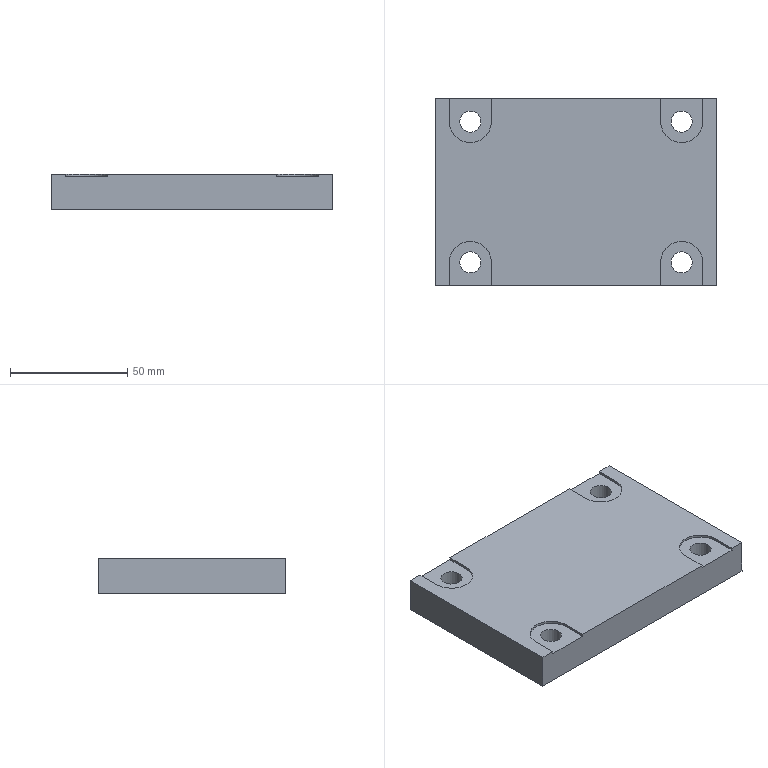Part | NX | 1 solid | 26 faces | box 120 x 80 x 15 mm | volume 139208 mm3 | plane 18 | cylinder 8 | commonest cylinder face diameters 9 x4 18 x4
STEP:
#1=CARTESIAN_POINT('',(-49.5,-30.,0.));
#2=VERTEX_POINT('',#1);
#3=CARTESIAN_POINT('',(-45.,-30.,0.));
#4=DIRECTION('',(0.,0.,1.));
#5=DIRECTION('',(-1.,0.,0.));
#6=AXIS2_PLACEMENT_3D('',#3,#4,#5);
#7=CIRCLE('',#6,4.5);
#8=EDGE_CURVE('',#2,#2,#7,.T.);
#9=ORIENTED_EDGE('',*,*,#8,.F.);
#10=EDGE_LOOP('',(#9));
#11=FACE_BOUND('',#10,.T.);
#12=CARTESIAN_POINT('',(-40.5,-30.,14.));
#13=VERTEX_POINT('',#12);
#14=CARTESIAN_POINT('',(-45.,-30.,14.));
#15=DIRECTION('',(0.,0.,1.));
#16=DIRECTION('',(1.,0.,0.));
#17=AXIS2_PLACEMENT_3D('',#14,#15,#16);
#18=CIRCLE('',#17,4.5);
#19=EDGE_CURVE('',#13,#13,#18,.F.);
#20=ORIENTED_EDGE('',*,*,#19,.F.);
#21=EDGE_LOOP('',(#20));
#22=FACE_BOUND('',#21,.T.);
#23=CARTESIAN_POINT('',(-45.,-30.,0.));
#24=DIRECTION('',(0.,0.,1.));
#25=DIRECTION('',(1.,0.,0.));
#26=AXIS2_PLACEMENT_3D('',#23,#24,#25);
#27=CYLINDRICAL_SURFACE('',#26,4.5);
#28=ADVANCED_FACE('',(#11,#22),#27,.F.);
#29=CARTESIAN_POINT('',(49.5,-30.,0.));
#30=VERTEX_POINT('',#29);
#31=CARTESIAN_POINT('',(45.,-30.,0.));
#32=DIRECTION('',(0.,0.,1.));
#33=DIRECTION('',(1.,0.,0.));
#34=AXIS2_PLACEMENT_3D('',#31,#32,#33);
#35=CIRCLE('',#34,4.5);
#36=EDGE_CURVE('',#30,#30,#35,.T.);
#37=ORIENTED_EDGE('',*,*,#36,.F.);
#38=EDGE_LOOP('',(#37));
#39=FACE_BOUND('',#38,.T.);
#40=CARTESIAN_POINT('',(49.5,-30.,14.));
#41=VERTEX_POINT('',#40);
#42=CARTESIAN_POINT('',(45.,-30.,14.));
#43=DIRECTION('',(0.,0.,1.));
#44=DIRECTION('',(1.,0.,0.));
#45=AXIS2_PLACEMENT_3D('',#42,#43,#44);
#46=CIRCLE('',#45,4.5);
#47=EDGE_CURVE('',#41,#41,#46,.F.);
#48=ORIENTED_EDGE('',*,*,#47,.F.);
#49=EDGE_LOOP('',(#48));
#50=FACE_BOUND('',#49,.T.);
#51=CARTESIAN_POINT('',(45.,-30.,0.));
#52=DIRECTION('',(0.,0.,1.));
#53=DIRECTION('',(1.,0.,0.));
#54=AXIS2_PLACEMENT_3D('',#51,#52,#53);
#55=CYLINDRICAL_SURFACE('',#54,4.5);
#56=ADVANCED_FACE('',(#39,#50),#55,.F.);
#57=CARTESIAN_POINT('',(40.5,30.,0.));
#58=VERTEX_POINT('',#57);
#59=CARTESIAN_POINT('',(45.,30.,0.));
#60=DIRECTION('',(0.,0.,1.));
#61=DIRECTION('',(-1.,0.,0.));
#62=AXIS2_PLACEMENT_3D('',#59,#60,#61);
#63=CIRCLE('',#62,4.5);
#64=EDGE_CURVE('',#58,#58,#63,.T.);
#65=ORIENTED_EDGE('',*,*,#64,.F.);
#66=EDGE_LOOP('',(#65));
#67=FACE_BOUND('',#66,.T.);
#68=CARTESIAN_POINT('',(49.5,30.,14.));
#69=VERTEX_POINT('',#68);
#70=CARTESIAN_POINT('',(45.,30.,14.));
#71=DIRECTION('',(0.,0.,1.));
#72=DIRECTION('',(1.,0.,0.));
#73=AXIS2_PLACEMENT_3D('',#70,#71,#72);
#74=CIRCLE('',#73,4.5);
#75=EDGE_CURVE('',#69,#69,#74,.F.);
#76=ORIENTED_EDGE('',*,*,#75,.F.);
#77=EDGE_LOOP('',(#76));
#78=FACE_BOUND('',#77,.T.);
#79=CARTESIAN_POINT('',(45.,30.,0.));
#80=DIRECTION('',(0.,0.,1.));
#81=DIRECTION('',(1.,0.,0.));
#82=AXIS2_PLACEMENT_3D('',#79,#80,#81);
#83=CYLINDRICAL_SURFACE('',#82,4.5);
#84=ADVANCED_FACE('',(#67,#78),#83,.F.);
#85=CARTESIAN_POINT('',(-40.5,30.,0.));
#86=VERTEX_POINT('',#85);
#87=CARTESIAN_POINT('',(-45.,30.,0.));
#88=DIRECTION('',(0.,0.,1.));
#89=DIRECTION('',(1.,0.,0.));
#90=AXIS2_PLACEMENT_3D('',#87,#88,#89);
#91=CIRCLE('',#90,4.5);
#92=EDGE_CURVE('',#86,#86,#91,.T.);
#93=ORIENTED_EDGE('',*,*,#92,.F.);
#94=EDGE_LOOP('',(#93));
#95=FACE_BOUND('',#94,.T.);
#96=CARTESIAN_POINT('',(-40.5,30.,14.));
#97=VERTEX_POINT('',#96);
#98=CARTESIAN_POINT('',(-45.,30.,14.));
#99=DIRECTION('',(0.,0.,1.));
#100=DIRECTION('',(1.,0.,0.));
#101=AXIS2_PLACEMENT_3D('',#98,#99,#100);
#102=CIRCLE('',#101,4.5);
#103=EDGE_CURVE('',#97,#97,#102,.F.);
#104=ORIENTED_EDGE('',*,*,#103,.F.);
#105=EDGE_LOOP('',(#104));
#106=FACE_BOUND('',#105,.T.);
#107=CARTESIAN_POINT('',(-45.,30.,0.));
#108=DIRECTION('',(0.,0.,1.));
#109=DIRECTION('',(1.,0.,0.));
#110=AXIS2_PLACEMENT_3D('',#107,#108,#109);
#111=CYLINDRICAL_SURFACE('',#110,4.5);
#112=ADVANCED_FACE('',(#95,#106),#111,.F.);
#113=CARTESIAN_POINT('',(60.,-40.,0.));
#114=VERTEX_POINT('',#113);
#115=CARTESIAN_POINT('',(60.,40.,0.));
#116=VERTEX_POINT('',#115);
#117=CARTESIAN_POINT('',(60.,-40.,0.));
#118=DIRECTION('',(0.,1.,0.));
#119=VECTOR('',#118,1000.);
#120=LINE('',#117,#119);
#121=EDGE_CURVE('',#114,#116,#120,.T.);
#122=ORIENTED_EDGE('',*,*,#121,.T.);
#123=CARTESIAN_POINT('',(60.,40.,15.));
#124=VERTEX_POINT('',#123);
#125=CARTESIAN_POINT('',(60.,40.,15.));
#126=DIRECTION('',(0.,0.,-1.));
#127=VECTOR('',#126,1000.);
#128=LINE('',#125,#127);
#129=EDGE_CURVE('',#124,#116,#128,.T.);
#130=ORIENTED_EDGE('',*,*,#129,.F.);
#131=CARTESIAN_POINT('',(60.,-40.,15.));
#132=VERTEX_POINT('',#131);
#133=CARTESIAN_POINT('',(60.,-40.,15.));
#134=DIRECTION('',(0.,1.,0.));
#135=VECTOR('',#134,1000.);
#136=LINE('',#133,#135);
#137=EDGE_CURVE('',#132,#124,#136,.T.);
#138=ORIENTED_EDGE('',*,*,#137,.F.);
#139=CARTESIAN_POINT('',(60.,-40.,15.));
#140=DIRECTION('',(0.,0.,-1.));
#141=VECTOR('',#140,1000.);
#142=LINE('',#139,#141);
#143=EDGE_CURVE('',#132,#114,#142,.T.);
#144=ORIENTED_EDGE('',*,*,#143,.T.);
#145=EDGE_LOOP('',(#122,#130,#138,#144));
#146=FACE_BOUND('',#145,.T.);
#147=CARTESIAN_POINT('',(60.,-40.,15.));
#148=DIRECTION('',(-1.,0.,0.));
#149=DIRECTION('',(0.,0.,1.));
#150=AXIS2_PLACEMENT_3D('',#147,#148,#149);
#151=PLANE('',#150);
#152=ADVANCED_FACE('',(#146),#151,.F.);
#153=CARTESIAN_POINT('',(36.,40.,15.));
#154=VERTEX_POINT('',#153);
#155=CARTESIAN_POINT('',(-36.,40.,15.));
#156=VERTEX_POINT('',#155);
#157=CARTESIAN_POINT('',(-60.,40.,15.));
#158=DIRECTION('',(-1.,0.,0.));
#159=VECTOR('',#158,1000.);
#160=LINE('',#157,#159);
#161=EDGE_CURVE('',#154,#156,#160,.T.);
#162=ORIENTED_EDGE('',*,*,#161,.F.);
#163=CARTESIAN_POINT('',(36.,40.,14.));
#164=VERTEX_POINT('',#163);
#165=CARTESIAN_POINT('',(36.,40.,14.));
#166=DIRECTION('',(0.,0.,1.));
#167=VECTOR('',#166,1000.);
#168=LINE('',#165,#167);
#169=EDGE_CURVE('',#164,#154,#168,.T.);
#170=ORIENTED_EDGE('',*,*,#169,.F.);
#171=CARTESIAN_POINT('',(54.,40.,14.));
#172=VERTEX_POINT('',#171);
#173=CARTESIAN_POINT('',(-60.,40.,14.));
#174=DIRECTION('',(-1.,0.,0.));
#175=VECTOR('',#174,1000.);
#176=LINE('',#173,#175);
#177=EDGE_CURVE('',#172,#164,#176,.T.);
#178=ORIENTED_EDGE('',*,*,#177,.F.);
#179=CARTESIAN_POINT('',(54.,40.,15.));
#180=VERTEX_POINT('',#179);
#181=CARTESIAN_POINT('',(54.,40.,14.));
#182=DIRECTION('',(0.,0.,1.));
#183=VECTOR('',#182,1000.);
#184=LINE('',#181,#183);
#185=EDGE_CURVE('',#172,#180,#184,.T.);
#186=ORIENTED_EDGE('',*,*,#185,.T.);
#187=CARTESIAN_POINT('',(-60.,40.,15.));
#188=DIRECTION('',(-1.,0.,0.));
#189=VECTOR('',#188,1000.);
#190=LINE('',#187,#189);
#191=EDGE_CURVE('',#124,#180,#190,.T.);
#192=ORIENTED_EDGE('',*,*,#191,.F.);
#193=ORIENTED_EDGE('',*,*,#129,.T.);
#194=CARTESIAN_POINT('',(-60.,40.,0.));
#195=VERTEX_POINT('',#194);
#196=CARTESIAN_POINT('',(-60.,40.,0.));
#197=DIRECTION('',(-1.,0.,0.));
#198=VECTOR('',#197,1000.);
#199=LINE('',#196,#198);
#200=EDGE_CURVE('',#116,#195,#199,.T.);
#201=ORIENTED_EDGE('',*,*,#200,.T.);
#202=CARTESIAN_POINT('',(-60.,40.,15.));
#203=VERTEX_POINT('',#202);
#204=CARTESIAN_POINT('',(-60.,40.,15.));
#205=DIRECTION('',(0.,0.,-1.));
#206=VECTOR('',#205,1000.);
#207=LINE('',#204,#206);
#208=EDGE_CURVE('',#203,#195,#207,.T.);
#209=ORIENTED_EDGE('',*,*,#208,.F.);
#210=CARTESIAN_POINT('',(-54.,40.,15.));
#211=VERTEX_POINT('',#210);
#212=CARTESIAN_POINT('',(-60.,40.,15.));
#213=DIRECTION('',(-1.,0.,0.));
#214=VECTOR('',#213,1000.);
#215=LINE('',#212,#214);
#216=EDGE_CURVE('',#211,#203,#215,.T.);
#217=ORIENTED_EDGE('',*,*,#216,.F.);
#218=CARTESIAN_POINT('',(-54.,40.,14.));
#219=VERTEX_POINT('',#218);
#220=CARTESIAN_POINT('',(-54.,40.,14.));
#221=DIRECTION('',(0.,0.,1.));
#222=VECTOR('',#221,1000.);
#223=LINE('',#220,#222);
#224=EDGE_CURVE('',#219,#211,#223,.T.);
#225=ORIENTED_EDGE('',*,*,#224,.F.);
#226=CARTESIAN_POINT('',(-36.,40.,14.));
#227=VERTEX_POINT('',#226);
#228=CARTESIAN_POINT('',(-60.,40.,14.));
#229=DIRECTION('',(-1.,0.,0.));
#230=VECTOR('',#229,1000.);
#231=LINE('',#228,#230);
#232=EDGE_CURVE('',#227,#219,#231,.T.);
#233=ORIENTED_EDGE('',*,*,#232,.F.);
#234=CARTESIAN_POINT('',(-36.,40.,14.));
#235=DIRECTION('',(0.,0.,1.));
#236=VECTOR('',#235,1000.);
#237=LINE('',#234,#236);
#238=EDGE_CURVE('',#227,#156,#237,.T.);
#239=ORIENTED_EDGE('',*,*,#238,.T.);
#240=EDGE_LOOP('',(#162,#170,#178,#186,#192,#193,#201,#209,#217,#225,#233,#239));
#241=FACE_BOUND('',#240,.T.);
#242=CARTESIAN_POINT('',(-60.,40.,15.));
#243=DIRECTION('',(0.,-1.,0.));
#244=DIRECTION('',(0.,0.,-1.));
#245=AXIS2_PLACEMENT_3D('',#242,#243,#244);
#246=PLANE('',#245);
#247=ADVANCED_FACE('',(#241),#246,.F.);
#248=CARTESIAN_POINT('',(-60.,-40.,0.));
#249=VERTEX_POINT('',#248);
#250=CARTESIAN_POINT('',(-60.,-40.,0.));
#251=DIRECTION('',(0.,-1.,0.));
#252=VECTOR('',#251,1000.);
#253=LINE('',#250,#252);
#254=EDGE_CURVE('',#195,#249,#253,.T.);
#255=ORIENTED_EDGE('',*,*,#254,.T.);
#256=CARTESIAN_POINT('',(-60.,-40.,15.));
#257=VERTEX_POINT('',#256);
#258=CARTESIAN_POINT('',(-60.,-40.,15.));
#259=DIRECTION('',(0.,0.,-1.));
#260=VECTOR('',#259,1000.);
#261=LINE('',#258,#260);
#262=EDGE_CURVE('',#257,#249,#261,.T.);
#263=ORIENTED_EDGE('',*,*,#262,.F.);
#264=CARTESIAN_POINT('',(-60.,-40.,15.));
#265=DIRECTION('',(0.,-1.,0.));
#266=VECTOR('',#265,1000.);
#267=LINE('',#264,#266);
#268=EDGE_CURVE('',#203,#257,#267,.T.);
#269=ORIENTED_EDGE('',*,*,#268,.F.);
#270=ORIENTED_EDGE('',*,*,#208,.T.);
#271=EDGE_LOOP('',(#255,#263,#269,#270));
#272=FACE_BOUND('',#271,.T.);
#273=CARTESIAN_POINT('',(-60.,-40.,15.));
#274=DIRECTION('',(1.,0.,0.));
#275=DIRECTION('',(0.,0.,-1.));
#276=AXIS2_PLACEMENT_3D('',#273,#274,#275);
#277=PLANE('',#276);
#278=ADVANCED_FACE('',(#272),#277,.F.);
#279=CARTESIAN_POINT('',(-36.,-40.,15.));
#280=VERTEX_POINT('',#279);
#281=CARTESIAN_POINT('',(36.,-40.,15.));
#282=VERTEX_POINT('',#281);
#283=CARTESIAN_POINT('',(-60.,-40.,15.));
#284=DIRECTION('',(1.,0.,0.));
#285=VECTOR('',#284,1000.);
#286=LINE('',#283,#285);
#287=EDGE_CURVE('',#280,#282,#286,.T.);
#288=ORIENTED_EDGE('',*,*,#287,.F.);
#289=CARTESIAN_POINT('',(-36.,-40.,14.));
#290=VERTEX_POINT('',#289);
#291=CARTESIAN_POINT('',(-36.,-40.,14.));
#292=DIRECTION('',(0.,0.,1.));
#293=VECTOR('',#292,1000.);
#294=LINE('',#291,#293);
#295=EDGE_CURVE('',#290,#280,#294,.T.);
#296=ORIENTED_EDGE('',*,*,#295,.F.);
#297=CARTESIAN_POINT('',(-54.,-40.,14.));
#298=VERTEX_POINT('',#297);
#299=CARTESIAN_POINT('',(-60.,-40.,14.));
#300=DIRECTION('',(1.,0.,0.));
#301=VECTOR('',#300,1000.);
#302=LINE('',#299,#301);
#303=EDGE_CURVE('',#298,#290,#302,.T.);
#304=ORIENTED_EDGE('',*,*,#303,.F.);
#305=CARTESIAN_POINT('',(-54.,-40.,15.));
#306=VERTEX_POINT('',#305);
#307=CARTESIAN_POINT('',(-54.,-40.,14.));
#308=DIRECTION('',(0.,0.,1.));
#309=VECTOR('',#308,1000.);
#310=LINE('',#307,#309);
#311=EDGE_CURVE('',#298,#306,#310,.T.);
#312=ORIENTED_EDGE('',*,*,#311,.T.);
#313=CARTESIAN_POINT('',(-60.,-40.,15.));
#314=DIRECTION('',(1.,0.,0.));
#315=VECTOR('',#314,1000.);
#316=LINE('',#313,#315);
#317=EDGE_CURVE('',#257,#306,#316,.T.);
#318=ORIENTED_EDGE('',*,*,#317,.F.);
#319=ORIENTED_EDGE('',*,*,#262,.T.);
#320=CARTESIAN_POINT('',(-60.,-40.,0.));
#321=DIRECTION('',(1.,0.,0.));
#322=VECTOR('',#321,1000.);
#323=LINE('',#320,#322);
#324=EDGE_CURVE('',#249,#114,#323,.T.);
#325=ORIENTED_EDGE('',*,*,#324,.T.);
#326=ORIENTED_EDGE('',*,*,#143,.F.);
#327=CARTESIAN_POINT('',(54.,-40.,15.));
#328=VERTEX_POINT('',#327);
#329=CARTESIAN_POINT('',(-60.,-40.,15.));
#330=DIRECTION('',(1.,0.,0.));
#331=VECTOR('',#330,1000.);
#332=LINE('',#329,#331);
#333=EDGE_CURVE('',#328,#132,#332,.T.);
#334=ORIENTED_EDGE('',*,*,#333,.F.);
#335=CARTESIAN_POINT('',(54.,-40.,14.));
#336=VERTEX_POINT('',#335);
#337=CARTESIAN_POINT('',(54.,-40.,14.));
#338=DIRECTION('',(0.,0.,1.));
#339=VECTOR('',#338,1000.);
#340=LINE('',#337,#339);
#341=EDGE_CURVE('',#336,#328,#340,.T.);
#342=ORIENTED_EDGE('',*,*,#341,.F.);
#343=CARTESIAN_POINT('',(36.,-40.,14.));
#344=VERTEX_POINT('',#343);
#345=CARTESIAN_POINT('',(-60.,-40.,14.));
#346=DIRECTION('',(1.,0.,0.));
#347=VECTOR('',#346,1000.);
#348=LINE('',#345,#347);
#349=EDGE_CURVE('',#344,#336,#348,.T.);
#350=ORIENTED_EDGE('',*,*,#349,.F.);
#351=CARTESIAN_POINT('',(36.,-40.,14.));
#352=DIRECTION('',(0.,0.,1.));
#353=VECTOR('',#352,1000.);
#354=LINE('',#351,#353);
#355=EDGE_CURVE('',#344,#282,#354,.T.);
#356=ORIENTED_EDGE('',*,*,#355,.T.);
#357=EDGE_LOOP('',(#288,#296,#304,#312,#318,#319,#325,#326,#334,#342,#350,#356));
#358=FACE_BOUND('',#357,.T.);
#359=CARTESIAN_POINT('',(-60.,-40.,15.));
#360=DIRECTION('',(0.,1.,0.));
#361=DIRECTION('',(0.,0.,1.));
#362=AXIS2_PLACEMENT_3D('',#359,#360,#361);
#363=PLANE('',#362);
#364=ADVANCED_FACE('',(#358),#363,.F.);
#365=CARTESIAN_POINT('',(-36.,-30.,15.));
#366=VERTEX_POINT('',#365);
#367=CARTESIAN_POINT('',(-54.,-30.,15.));
#368=VERTEX_POINT('',#367);
#369=CARTESIAN_POINT('',(-45.,-30.,15.));
#370=DIRECTION('',(0.,0.,1.));
#371=DIRECTION('',(1.,0.,0.));
#372=AXIS2_PLACEMENT_3D('',#369,#370,#371);
#373=CIRCLE('',#372,9.);
#374=EDGE_CURVE('',#366,#368,#373,.T.);
#375=ORIENTED_EDGE('',*,*,#374,.F.);
#376=CARTESIAN_POINT('',(-36.,-30.,15.));
#377=DIRECTION('',(0.,1.,0.));
#378=VECTOR('',#377,1000.);
#379=LINE('',#376,#378);
#380=EDGE_CURVE('',#280,#366,#379,.T.);
#381=ORIENTED_EDGE('',*,*,#380,.F.);
#382=ORIENTED_EDGE('',*,*,#287,.T.);
#383=CARTESIAN_POINT('',(36.,-30.,15.));
#384=VERTEX_POINT('',#383);
#385=CARTESIAN_POINT('',(36.,-30.,15.));
#386=DIRECTION('',(0.,-1.,0.));
#387=VECTOR('',#386,1000.);
#388=LINE('',#385,#387);
#389=EDGE_CURVE('',#384,#282,#388,.T.);
#390=ORIENTED_EDGE('',*,*,#389,.F.);
#391=CARTESIAN_POINT('',(54.,-30.,15.));
#392=VERTEX_POINT('',#391);
#393=CARTESIAN_POINT('',(45.,-30.,15.));
#394=DIRECTION('',(0.,0.,1.));
#395=DIRECTION('',(1.,0.,0.));
#396=AXIS2_PLACEMENT_3D('',#393,#394,#395);
#397=CIRCLE('',#396,9.);
#398=EDGE_CURVE('',#392,#384,#397,.T.);
#399=ORIENTED_EDGE('',*,*,#398,.F.);
#400=CARTESIAN_POINT('',(54.,-30.,15.));
#401=DIRECTION('',(0.,1.,0.));
#402=VECTOR('',#401,1000.);
#403=LINE('',#400,#402);
#404=EDGE_CURVE('',#328,#392,#403,.T.);
#405=ORIENTED_EDGE('',*,*,#404,.F.);
#406=ORIENTED_EDGE('',*,*,#333,.T.);
#407=ORIENTED_EDGE('',*,*,#137,.T.);
#408=ORIENTED_EDGE('',*,*,#191,.T.);
#409=CARTESIAN_POINT('',(54.,30.,15.));
#410=VERTEX_POINT('',#409);
#411=CARTESIAN_POINT('',(54.,30.,15.));
#412=DIRECTION('',(0.,1.,0.));
#413=VECTOR('',#412,1000.);
#414=LINE('',#411,#413);
#415=EDGE_CURVE('',#410,#180,#414,.T.);
#416=ORIENTED_EDGE('',*,*,#415,.F.);
#417=CARTESIAN_POINT('',(36.,30.,15.));
#418=VERTEX_POINT('',#417);
#419=CARTESIAN_POINT('',(45.,30.,15.));
#420=DIRECTION('',(0.,0.,1.));
#421=DIRECTION('',(1.,0.,0.));
#422=AXIS2_PLACEMENT_3D('',#419,#420,#421);
#423=CIRCLE('',#422,9.);
#424=EDGE_CURVE('',#418,#410,#423,.T.);
#425=ORIENTED_EDGE('',*,*,#424,.F.);
#426=CARTESIAN_POINT('',(36.,30.,15.));
#427=DIRECTION('',(0.,-1.,0.));
#428=VECTOR('',#427,1000.);
#429=LINE('',#426,#428);
#430=EDGE_CURVE('',#154,#418,#429,.T.);
#431=ORIENTED_EDGE('',*,*,#430,.F.);
#432=ORIENTED_EDGE('',*,*,#161,.T.);
#433=CARTESIAN_POINT('',(-36.,30.,15.));
#434=VERTEX_POINT('',#433);
#435=CARTESIAN_POINT('',(-36.,30.,15.));
#436=DIRECTION('',(0.,1.,0.));
#437=VECTOR('',#436,1000.);
#438=LINE('',#435,#437);
#439=EDGE_CURVE('',#434,#156,#438,.T.);
#440=ORIENTED_EDGE('',*,*,#439,.F.);
#441=CARTESIAN_POINT('',(-54.,30.,15.));
#442=VERTEX_POINT('',#441);
#443=CARTESIAN_POINT('',(-45.,30.,15.));
#444=DIRECTION('',(0.,0.,1.));
#445=DIRECTION('',(1.,0.,0.));
#446=AXIS2_PLACEMENT_3D('',#443,#444,#445);
#447=CIRCLE('',#446,9.);
#448=EDGE_CURVE('',#442,#434,#447,.T.);
#449=ORIENTED_EDGE('',*,*,#448,.F.);
#450=CARTESIAN_POINT('',(-54.,30.,15.));
#451=DIRECTION('',(0.,-1.,0.));
#452=VECTOR('',#451,1000.);
#453=LINE('',#450,#452);
#454=EDGE_CURVE('',#211,#442,#453,.T.);
#455=ORIENTED_EDGE('',*,*,#454,.F.);
#456=ORIENTED_EDGE('',*,*,#216,.T.);
#457=ORIENTED_EDGE('',*,*,#268,.T.);
#458=ORIENTED_EDGE('',*,*,#317,.T.);
#459=CARTESIAN_POINT('',(-54.,-30.,15.));
#460=DIRECTION('',(0.,-1.,0.));
#461=VECTOR('',#460,1000.);
#462=LINE('',#459,#461);
#463=EDGE_CURVE('',#368,#306,#462,.T.);
#464=ORIENTED_EDGE('',*,*,#463,.F.);
#465=EDGE_LOOP('',(#375,#381,#382,#390,#399,#405,#406,#407,#408,#416,#425,#431,#432,#440,#449,#455,#456,#457,#458,#464));
#466=FACE_BOUND('',#465,.T.);
#467=CARTESIAN_POINT('',(0.,0.,15.));
#468=DIRECTION('',(0.,0.,-1.));
#469=DIRECTION('',(-1.,0.,0.));
#470=AXIS2_PLACEMENT_3D('',#467,#468,#469);
#471=PLANE('',#470);
#472=ADVANCED_FACE('',(#466),#471,.F.);
#473=ORIENTED_EDGE('',*,*,#8,.T.);
#474=EDGE_LOOP('',(#473));
#475=FACE_BOUND('',#474,.T.);
#476=ORIENTED_EDGE('',*,*,#36,.T.);
#477=EDGE_LOOP('',(#476));
#478=FACE_BOUND('',#477,.T.);
#479=ORIENTED_EDGE('',*,*,#64,.T.);
#480=EDGE_LOOP('',(#479));
#481=FACE_BOUND('',#480,.T.);
#482=ORIENTED_EDGE('',*,*,#92,.T.);
#483=EDGE_LOOP('',(#482));
#484=FACE_BOUND('',#483,.T.);
#485=ORIENTED_EDGE('',*,*,#121,.F.);
#486=ORIENTED_EDGE('',*,*,#324,.F.);
#487=ORIENTED_EDGE('',*,*,#254,.F.);
#488=ORIENTED_EDGE('',*,*,#200,.F.);
#489=EDGE_LOOP('',(#485,#486,#487,#488));
#490=FACE_BOUND('',#489,.T.);
#491=CARTESIAN_POINT('',(0.,0.,0.));
#492=DIRECTION('',(0.,0.,-1.));
#493=DIRECTION('',(-1.,0.,0.));
#494=AXIS2_PLACEMENT_3D('',#491,#492,#493);
#495=PLANE('',#494);
#496=ADVANCED_FACE('',(#475,#478,#481,#484,#490),#495,.T.);
#497=ORIENTED_EDGE('',*,*,#103,.T.);
#498=EDGE_LOOP('',(#497));
#499=FACE_BOUND('',#498,.T.);
#500=ORIENTED_EDGE('',*,*,#232,.T.);
#501=CARTESIAN_POINT('',(-54.,30.,14.));
#502=VERTEX_POINT('',#501);
#503=CARTESIAN_POINT('',(-54.,30.,14.));
#504=DIRECTION('',(0.,-1.,0.));
#505=VECTOR('',#504,1000.);
#506=LINE('',#503,#505);
#507=EDGE_CURVE('',#219,#502,#506,.T.);
#508=ORIENTED_EDGE('',*,*,#507,.T.);
#509=CARTESIAN_POINT('',(-36.,30.,14.));
#510=VERTEX_POINT('',#509);
#511=CARTESIAN_POINT('',(-45.,30.,14.));
#512=DIRECTION('',(0.,0.,1.));
#513=DIRECTION('',(1.,0.,0.));
#514=AXIS2_PLACEMENT_3D('',#511,#512,#513);
#515=CIRCLE('',#514,9.);
#516=EDGE_CURVE('',#502,#510,#515,.T.);
#517=ORIENTED_EDGE('',*,*,#516,.T.);
#518=CARTESIAN_POINT('',(-36.,30.,14.));
#519=DIRECTION('',(0.,1.,0.));
#520=VECTOR('',#519,1000.);
#521=LINE('',#518,#520);
#522=EDGE_CURVE('',#510,#227,#521,.T.);
#523=ORIENTED_EDGE('',*,*,#522,.T.);
#524=EDGE_LOOP('',(#500,#508,#517,#523));
#525=FACE_BOUND('',#524,.T.);
#526=CARTESIAN_POINT('',(-45.,30.,14.));
#527=DIRECTION('',(0.,0.,1.));
#528=DIRECTION('',(1.,0.,0.));
#529=AXIS2_PLACEMENT_3D('',#526,#527,#528);
#530=PLANE('',#529);
#531=ADVANCED_FACE('',(#499,#525),#530,.T.);
#532=ORIENTED_EDGE('',*,*,#448,.T.);
#533=CARTESIAN_POINT('',(-36.,30.,14.));
#534=DIRECTION('',(0.,0.,1.));
#535=VECTOR('',#534,1000.);
#536=LINE('',#533,#535);
#537=EDGE_CURVE('',#510,#434,#536,.T.);
#538=ORIENTED_EDGE('',*,*,#537,.F.);
#539=ORIENTED_EDGE('',*,*,#516,.F.);
#540=CARTESIAN_POINT('',(-54.,30.,14.));
#541=DIRECTION('',(0.,0.,1.));
#542=VECTOR('',#541,1000.);
#543=LINE('',#540,#542);
#544=EDGE_CURVE('',#502,#442,#543,.T.);
#545=ORIENTED_EDGE('',*,*,#544,.T.);
#546=EDGE_LOOP('',(#532,#538,#539,#545));
#547=FACE_BOUND('',#546,.T.);
#548=CARTESIAN_POINT('',(-45.,30.,14.));
#549=DIRECTION('',(0.,0.,1.));
#550=DIRECTION('',(1.,0.,0.));
#551=AXIS2_PLACEMENT_3D('',#548,#549,#550);
#552=CYLINDRICAL_SURFACE('',#551,9.);
#553=ADVANCED_FACE('',(#547),#552,.F.);
#554=ORIENTED_EDGE('',*,*,#454,.T.);
#555=ORIENTED_EDGE('',*,*,#544,.F.);
#556=ORIENTED_EDGE('',*,*,#507,.F.);
#557=ORIENTED_EDGE('',*,*,#224,.T.);
#558=EDGE_LOOP('',(#554,#555,#556,#557));
#559=FACE_BOUND('',#558,.T.);
#560=CARTESIAN_POINT('',(-54.,30.,14.));
#561=DIRECTION('',(-1.,0.,0.));
#562=DIRECTION('',(0.,0.,1.));
#563=AXIS2_PLACEMENT_3D('',#560,#561,#562);
#564=PLANE('',#563);
#565=ADVANCED_FACE('',(#559),#564,.F.);
#566=ORIENTED_EDGE('',*,*,#439,.T.);
#567=ORIENTED_EDGE('',*,*,#238,.F.);
#568=ORIENTED_EDGE('',*,*,#522,.F.);
#569=ORIENTED_EDGE('',*,*,#537,.T.);
#570=EDGE_LOOP('',(#566,#567,#568,#569));
#571=FACE_BOUND('',#570,.T.);
#572=CARTESIAN_POINT('',(-36.,30.,14.));
#573=DIRECTION('',(1.,0.,0.));
#574=DIRECTION('',(0.,0.,-1.));
#575=AXIS2_PLACEMENT_3D('',#572,#573,#574);
#576=PLANE('',#575);
#577=ADVANCED_FACE('',(#571),#576,.F.);
#578=ORIENTED_EDGE('',*,*,#75,.T.);
#579=EDGE_LOOP('',(#578));
#580=FACE_BOUND('',#579,.T.);
#581=ORIENTED_EDGE('',*,*,#177,.T.);
#582=CARTESIAN_POINT('',(36.,30.,14.));
#583=VERTEX_POINT('',#582);
#584=CARTESIAN_POINT('',(36.,30.,14.));
#585=DIRECTION('',(0.,-1.,0.));
#586=VECTOR('',#585,1000.);
#587=LINE('',#584,#586);
#588=EDGE_CURVE('',#164,#583,#587,.T.);
#589=ORIENTED_EDGE('',*,*,#588,.T.);
#590=CARTESIAN_POINT('',(54.,30.,14.));
#591=VERTEX_POINT('',#590);
#592=CARTESIAN_POINT('',(45.,30.,14.));
#593=DIRECTION('',(0.,0.,1.));
#594=DIRECTION('',(1.,0.,0.));
#595=AXIS2_PLACEMENT_3D('',#592,#593,#594);
#596=CIRCLE('',#595,9.);
#597=EDGE_CURVE('',#583,#591,#596,.T.);
#598=ORIENTED_EDGE('',*,*,#597,.T.);
#599=CARTESIAN_POINT('',(54.,30.,14.));
#600=DIRECTION('',(0.,1.,0.));
#601=VECTOR('',#600,1000.);
#602=LINE('',#599,#601);
#603=EDGE_CURVE('',#591,#172,#602,.T.);
#604=ORIENTED_EDGE('',*,*,#603,.T.);
#605=EDGE_LOOP('',(#581,#589,#598,#604));
#606=FACE_BOUND('',#605,.T.);
#607=CARTESIAN_POINT('',(45.,30.,14.));
#608=DIRECTION('',(0.,0.,1.));
#609=DIRECTION('',(1.,0.,0.));
#610=AXIS2_PLACEMENT_3D('',#607,#608,#609);
#611=PLANE('',#610);
#612=ADVANCED_FACE('',(#580,#606),#611,.T.);
#613=ORIENTED_EDGE('',*,*,#424,.T.);
#614=CARTESIAN_POINT('',(54.,30.,14.));
#615=DIRECTION('',(0.,0.,1.));
#616=VECTOR('',#615,1000.);
#617=LINE('',#614,#616);
#618=EDGE_CURVE('',#591,#410,#617,.T.);
#619=ORIENTED_EDGE('',*,*,#618,.F.);
#620=ORIENTED_EDGE('',*,*,#597,.F.);
#621=CARTESIAN_POINT('',(36.,30.,14.));
#622=DIRECTION('',(0.,0.,1.));
#623=VECTOR('',#622,1000.);
#624=LINE('',#621,#623);
#625=EDGE_CURVE('',#583,#418,#624,.T.);
#626=ORIENTED_EDGE('',*,*,#625,.T.);
#627=EDGE_LOOP('',(#613,#619,#620,#626));
#628=FACE_BOUND('',#627,.T.);
#629=CARTESIAN_POINT('',(45.,30.,14.));
#630=DIRECTION('',(0.,0.,1.));
#631=DIRECTION('',(1.,0.,0.));
#632=AXIS2_PLACEMENT_3D('',#629,#630,#631);
#633=CYLINDRICAL_SURFACE('',#632,9.);
#634=ADVANCED_FACE('',(#628),#633,.F.);
#635=ORIENTED_EDGE('',*,*,#430,.T.);
#636=ORIENTED_EDGE('',*,*,#625,.F.);
#637=ORIENTED_EDGE('',*,*,#588,.F.);
#638=ORIENTED_EDGE('',*,*,#169,.T.);
#639=EDGE_LOOP('',(#635,#636,#637,#638));
#640=FACE_BOUND('',#639,.T.);
#641=CARTESIAN_POINT('',(36.,30.,14.));
#642=DIRECTION('',(-1.,0.,0.));
#643=DIRECTION('',(0.,0.,1.));
#644=AXIS2_PLACEMENT_3D('',#641,#642,#643);
#645=PLANE('',#644);
#646=ADVANCED_FACE('',(#640),#645,.F.);
#647=ORIENTED_EDGE('',*,*,#415,.T.);
#648=ORIENTED_EDGE('',*,*,#185,.F.);
#649=ORIENTED_EDGE('',*,*,#603,.F.);
#650=ORIENTED_EDGE('',*,*,#618,.T.);
#651=EDGE_LOOP('',(#647,#648,#649,#650));
#652=FACE_BOUND('',#651,.T.);
#653=CARTESIAN_POINT('',(54.,30.,14.));
#654=DIRECTION('',(1.,0.,0.));
#655=DIRECTION('',(0.,0.,-1.));
#656=AXIS2_PLACEMENT_3D('',#653,#654,#655);
#657=PLANE('',#656);
#658=ADVANCED_FACE('',(#652),#657,.F.);
#659=ORIENTED_EDGE('',*,*,#47,.T.);
#660=EDGE_LOOP('',(#659));
#661=FACE_BOUND('',#660,.T.);
#662=ORIENTED_EDGE('',*,*,#349,.T.);
#663=CARTESIAN_POINT('',(54.,-30.,14.));
#664=VERTEX_POINT('',#663);
#665=CARTESIAN_POINT('',(54.,-30.,14.));
#666=DIRECTION('',(0.,1.,0.));
#667=VECTOR('',#666,1000.);
#668=LINE('',#665,#667);
#669=EDGE_CURVE('',#336,#664,#668,.T.);
#670=ORIENTED_EDGE('',*,*,#669,.T.);
#671=CARTESIAN_POINT('',(36.,-30.,14.));
#672=VERTEX_POINT('',#671);
#673=CARTESIAN_POINT('',(45.,-30.,14.));
#674=DIRECTION('',(0.,0.,1.));
#675=DIRECTION('',(1.,0.,0.));
#676=AXIS2_PLACEMENT_3D('',#673,#674,#675);
#677=CIRCLE('',#676,9.);
#678=EDGE_CURVE('',#664,#672,#677,.T.);
#679=ORIENTED_EDGE('',*,*,#678,.T.);
#680=CARTESIAN_POINT('',(36.,-30.,14.));
#681=DIRECTION('',(0.,-1.,0.));
#682=VECTOR('',#681,1000.);
#683=LINE('',#680,#682);
#684=EDGE_CURVE('',#672,#344,#683,.T.);
#685=ORIENTED_EDGE('',*,*,#684,.T.);
#686=EDGE_LOOP('',(#662,#670,#679,#685));
#687=FACE_BOUND('',#686,.T.);
#688=CARTESIAN_POINT('',(45.,-30.,14.));
#689=DIRECTION('',(0.,0.,1.));
#690=DIRECTION('',(1.,0.,0.));
#691=AXIS2_PLACEMENT_3D('',#688,#689,#690);
#692=PLANE('',#691);
#693=ADVANCED_FACE('',(#661,#687),#692,.T.);
#694=ORIENTED_EDGE('',*,*,#398,.T.);
#695=CARTESIAN_POINT('',(36.,-30.,14.));
#696=DIRECTION('',(0.,0.,1.));
#697=VECTOR('',#696,1000.);
#698=LINE('',#695,#697);
#699=EDGE_CURVE('',#672,#384,#698,.T.);
#700=ORIENTED_EDGE('',*,*,#699,.F.);
#701=ORIENTED_EDGE('',*,*,#678,.F.);
#702=CARTESIAN_POINT('',(54.,-30.,14.));
#703=DIRECTION('',(0.,0.,1.));
#704=VECTOR('',#703,1000.);
#705=LINE('',#702,#704);
#706=EDGE_CURVE('',#664,#392,#705,.T.);
#707=ORIENTED_EDGE('',*,*,#706,.T.);
#708=EDGE_LOOP('',(#694,#700,#701,#707));
#709=FACE_BOUND('',#708,.T.);
#710=CARTESIAN_POINT('',(45.,-30.,14.));
#711=DIRECTION('',(0.,0.,1.));
#712=DIRECTION('',(1.,0.,0.));
#713=AXIS2_PLACEMENT_3D('',#710,#711,#712);
#714=CYLINDRICAL_SURFACE('',#713,9.);
#715=ADVANCED_FACE('',(#709),#714,.F.);
#716=ORIENTED_EDGE('',*,*,#404,.T.);
#717=ORIENTED_EDGE('',*,*,#706,.F.);
#718=ORIENTED_EDGE('',*,*,#669,.F.);
#719=ORIENTED_EDGE('',*,*,#341,.T.);
#720=EDGE_LOOP('',(#716,#717,#718,#719));
#721=FACE_BOUND('',#720,.T.);
#722=CARTESIAN_POINT('',(54.,-30.,14.));
#723=DIRECTION('',(1.,0.,0.));
#724=DIRECTION('',(0.,0.,-1.));
#725=AXIS2_PLACEMENT_3D('',#722,#723,#724);
#726=PLANE('',#725);
#727=ADVANCED_FACE('',(#721),#726,.F.);
#728=ORIENTED_EDGE('',*,*,#389,.T.);
#729=ORIENTED_EDGE('',*,*,#355,.F.);
#730=ORIENTED_EDGE('',*,*,#684,.F.);
#731=ORIENTED_EDGE('',*,*,#699,.T.);
#732=EDGE_LOOP('',(#728,#729,#730,#731));
#733=FACE_BOUND('',#732,.T.);
#734=CARTESIAN_POINT('',(36.,-30.,14.));
#735=DIRECTION('',(-1.,0.,0.));
#736=DIRECTION('',(0.,0.,1.));
#737=AXIS2_PLACEMENT_3D('',#734,#735,#736);
#738=PLANE('',#737);
#739=ADVANCED_FACE('',(#733),#738,.F.);
#740=ORIENTED_EDGE('',*,*,#19,.T.);
#741=EDGE_LOOP('',(#740));
#742=FACE_BOUND('',#741,.T.);
#743=ORIENTED_EDGE('',*,*,#303,.T.);
#744=CARTESIAN_POINT('',(-36.,-30.,14.));
#745=VERTEX_POINT('',#744);
#746=CARTESIAN_POINT('',(-36.,-30.,14.));
#747=DIRECTION('',(0.,1.,0.));
#748=VECTOR('',#747,1000.);
#749=LINE('',#746,#748);
#750=EDGE_CURVE('',#290,#745,#749,.T.);
#751=ORIENTED_EDGE('',*,*,#750,.T.);
#752=CARTESIAN_POINT('',(-54.,-30.,14.));
#753=VERTEX_POINT('',#752);
#754=CARTESIAN_POINT('',(-45.,-30.,14.));
#755=DIRECTION('',(0.,0.,1.));
#756=DIRECTION('',(1.,0.,0.));
#757=AXIS2_PLACEMENT_3D('',#754,#755,#756);
#758=CIRCLE('',#757,9.);
#759=EDGE_CURVE('',#745,#753,#758,.T.);
#760=ORIENTED_EDGE('',*,*,#759,.T.);
#761=CARTESIAN_POINT('',(-54.,-30.,14.));
#762=DIRECTION('',(0.,-1.,0.));
#763=VECTOR('',#762,1000.);
#764=LINE('',#761,#763);
#765=EDGE_CURVE('',#753,#298,#764,.T.);
#766=ORIENTED_EDGE('',*,*,#765,.T.);
#767=EDGE_LOOP('',(#743,#751,#760,#766));
#768=FACE_BOUND('',#767,.T.);
#769=CARTESIAN_POINT('',(-45.,-30.,14.));
#770=DIRECTION('',(0.,0.,1.));
#771=DIRECTION('',(1.,0.,0.));
#772=AXIS2_PLACEMENT_3D('',#769,#770,#771);
#773=PLANE('',#772);
#774=ADVANCED_FACE('',(#742,#768),#773,.T.);
#775=ORIENTED_EDGE('',*,*,#374,.T.);
#776=CARTESIAN_POINT('',(-54.,-30.,14.));
#777=DIRECTION('',(0.,0.,1.));
#778=VECTOR('',#777,1000.);
#779=LINE('',#776,#778);
#780=EDGE_CURVE('',#753,#368,#779,.T.);
#781=ORIENTED_EDGE('',*,*,#780,.F.);
#782=ORIENTED_EDGE('',*,*,#759,.F.);
#783=CARTESIAN_POINT('',(-36.,-30.,14.));
#784=DIRECTION('',(0.,0.,1.));
#785=VECTOR('',#784,1000.);
#786=LINE('',#783,#785);
#787=EDGE_CURVE('',#745,#366,#786,.T.);
#788=ORIENTED_EDGE('',*,*,#787,.T.);
#789=EDGE_LOOP('',(#775,#781,#782,#788));
#790=FACE_BOUND('',#789,.T.);
#791=CARTESIAN_POINT('',(-45.,-30.,14.));
#792=DIRECTION('',(0.,0.,1.));
#793=DIRECTION('',(1.,0.,0.));
#794=AXIS2_PLACEMENT_3D('',#791,#792,#793);
#795=CYLINDRICAL_SURFACE('',#794,9.);
#796=ADVANCED_FACE('',(#790),#795,.F.);
#797=ORIENTED_EDGE('',*,*,#380,.T.);
#798=ORIENTED_EDGE('',*,*,#787,.F.);
#799=ORIENTED_EDGE('',*,*,#750,.F.);
#800=ORIENTED_EDGE('',*,*,#295,.T.);
#801=EDGE_LOOP('',(#797,#798,#799,#800));
#802=FACE_BOUND('',#801,.T.);
#803=CARTESIAN_POINT('',(-36.,-30.,14.));
#804=DIRECTION('',(1.,0.,0.));
#805=DIRECTION('',(0.,0.,-1.));
#806=AXIS2_PLACEMENT_3D('',#803,#804,#805);
#807=PLANE('',#806);
#808=ADVANCED_FACE('',(#802),#807,.F.);
#809=ORIENTED_EDGE('',*,*,#463,.T.);
#810=ORIENTED_EDGE('',*,*,#311,.F.);
#811=ORIENTED_EDGE('',*,*,#765,.F.);
#812=ORIENTED_EDGE('',*,*,#780,.T.);
#813=EDGE_LOOP('',(#809,#810,#811,#812));
#814=FACE_BOUND('',#813,.T.);
#815=CARTESIAN_POINT('',(-54.,-30.,14.));
#816=DIRECTION('',(-1.,0.,0.));
#817=DIRECTION('',(0.,0.,1.));
#818=AXIS2_PLACEMENT_3D('',#815,#816,#817);
#819=PLANE('',#818);
#820=ADVANCED_FACE('',(#814),#819,.F.);
#821=CLOSED_SHELL('',(#28,#56,#84,#112,#152,#247,#278,#364,#472,#496,#531,#553,#565,#577,#612,#634,#646,#658,#693,#715,#727,#739,#774,#796,#808,#820));
#822=MANIFOLD_SOLID_BREP('',#821);
#823=(LENGTH_UNIT()NAMED_UNIT(*)SI_UNIT(.MILLI.,.METRE.));
#824=UNCERTAINTY_MEASURE_WITH_UNIT(LENGTH_MEASURE(0.00001),#823,'','');
#825=(NAMED_UNIT(*)PLANE_ANGLE_UNIT()SI_UNIT($,.RADIAN.));
#826=(NAMED_UNIT(*)SI_UNIT($,.STERADIAN.)SOLID_ANGLE_UNIT());
#827=(GEOMETRIC_REPRESENTATION_CONTEXT(3)GLOBAL_UNCERTAINTY_ASSIGNED_CONTEXT((#824))GLOBAL_UNIT_ASSIGNED_CONTEXT((#823,#825,#826))REPRESENTATION_CONTEXT('',''));
#828=ADVANCED_BREP_SHAPE_REPRESENTATION('',(#822),#827);